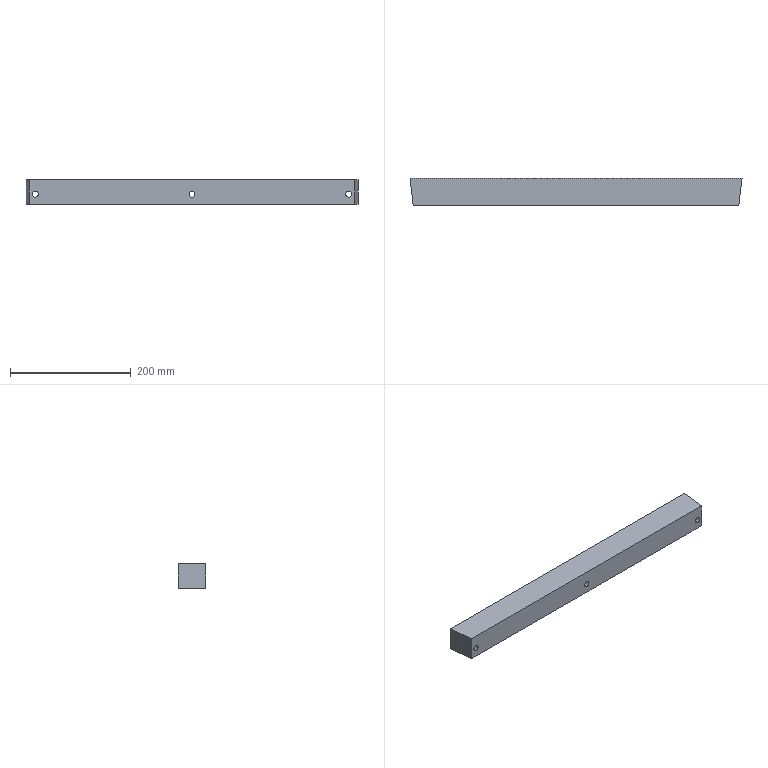Part | SolidWorks | features Extrusion 1, ICE 1 | 1 solid | 12 faces | box 550.66 x 45.55 x 40.5 mm | volume 995279 mm3 | cylinder 6 | plane 6 | commonest cylinder face diameters 10 x6
STEP:
#1=CARTESIAN_POINT('',(535.33,-45.55,-8.62));
#2=VERTEX_POINT('',#1);
#3=CARTESIAN_POINT('',(535.33,-45.55,1.38));
#4=VERTEX_POINT('',#3);
#5=CARTESIAN_POINT('',(535.33,-45.55,-3.62));
#6=DIRECTION('',(0.,1.,0.));
#7=DIRECTION('',(0.,0.,1.));
#8=AXIS2_PLACEMENT_3D('',#5,#6,#7);
#9=CIRCLE('',#8,5.);
#10=EDGE_CURVE('',#2,#4,#9,.T.);
#11=ORIENTED_EDGE('',*,*,#10,.F.);
#12=CARTESIAN_POINT('',(535.33,0.,-8.62));
#13=VERTEX_POINT('',#12);
#14=CARTESIAN_POINT('',(535.33,-52.5,-8.62));
#15=DIRECTION('',(0.,1.,0.));
#16=VECTOR('',#15,1000.);
#17=LINE('',#14,#16);
#18=EDGE_CURVE('',#2,#13,#17,.T.);
#19=ORIENTED_EDGE('',*,*,#18,.T.);
#20=CARTESIAN_POINT('',(535.33,0.,1.38));
#21=VERTEX_POINT('',#20);
#22=CARTESIAN_POINT('',(535.33,0.,-3.62));
#23=DIRECTION('',(0.,1.,0.));
#24=DIRECTION('',(0.,0.,1.));
#25=AXIS2_PLACEMENT_3D('',#22,#23,#24);
#26=CIRCLE('',#25,5.);
#27=EDGE_CURVE('',#13,#21,#26,.T.);
#28=ORIENTED_EDGE('',*,*,#27,.T.);
#29=CARTESIAN_POINT('',(535.33,-52.5,1.38));
#30=DIRECTION('',(0.,1.,0.));
#31=VECTOR('',#30,1000.);
#32=LINE('',#29,#31);
#33=EDGE_CURVE('',#4,#21,#32,.T.);
#34=ORIENTED_EDGE('',*,*,#33,.F.);
#35=EDGE_LOOP('',(#11,#19,#28,#34));
#36=FACE_OUTER_BOUND('',#35,.T.);
#37=CARTESIAN_POINT('',(535.33,-52.5,-3.62));
#38=DIRECTION('',(0.,1.,0.));
#39=DIRECTION('',(0.,0.,1.));
#40=AXIS2_PLACEMENT_3D('',#37,#38,#39);
#41=CYLINDRICAL_SURFACE('',#40,5.);
#42=ADVANCED_FACE('',(#36),#41,.F.);
#43=CARTESIAN_POINT('',(275.33,-45.55,-8.62));
#44=VERTEX_POINT('',#43);
#45=CARTESIAN_POINT('',(275.33,-45.55,1.38));
#46=VERTEX_POINT('',#45);
#47=CARTESIAN_POINT('',(275.33,-45.55,-3.62));
#48=DIRECTION('',(0.,1.,0.));
#49=DIRECTION('',(0.,0.,1.));
#50=AXIS2_PLACEMENT_3D('',#47,#48,#49);
#51=CIRCLE('',#50,5.);
#52=EDGE_CURVE('',#44,#46,#51,.T.);
#53=ORIENTED_EDGE('',*,*,#52,.F.);
#54=CARTESIAN_POINT('',(275.33,0.,-8.62));
#55=VERTEX_POINT('',#54);
#56=CARTESIAN_POINT('',(275.33,-52.5,-8.62));
#57=DIRECTION('',(0.,1.,0.));
#58=VECTOR('',#57,1000.);
#59=LINE('',#56,#58);
#60=EDGE_CURVE('',#44,#55,#59,.T.);
#61=ORIENTED_EDGE('',*,*,#60,.T.);
#62=CARTESIAN_POINT('',(275.33,0.,1.38));
#63=VERTEX_POINT('',#62);
#64=CARTESIAN_POINT('',(275.33,0.,-3.62));
#65=DIRECTION('',(0.,1.,0.));
#66=DIRECTION('',(0.,0.,1.));
#67=AXIS2_PLACEMENT_3D('',#64,#65,#66);
#68=CIRCLE('',#67,5.);
#69=EDGE_CURVE('',#55,#63,#68,.T.);
#70=ORIENTED_EDGE('',*,*,#69,.T.);
#71=CARTESIAN_POINT('',(275.33,-52.5,1.38));
#72=DIRECTION('',(0.,1.,0.));
#73=VECTOR('',#72,1000.);
#74=LINE('',#71,#73);
#75=EDGE_CURVE('',#46,#63,#74,.T.);
#76=ORIENTED_EDGE('',*,*,#75,.F.);
#77=EDGE_LOOP('',(#53,#61,#70,#76));
#78=FACE_OUTER_BOUND('',#77,.T.);
#79=CARTESIAN_POINT('',(275.33,-52.5,-3.62));
#80=DIRECTION('',(0.,1.,0.));
#81=DIRECTION('',(0.,0.,1.));
#82=AXIS2_PLACEMENT_3D('',#79,#80,#81);
#83=CYLINDRICAL_SURFACE('',#82,5.);
#84=ADVANCED_FACE('',(#78),#83,.F.);
#85=CARTESIAN_POINT('',(15.33,-45.55,-8.62));
#86=VERTEX_POINT('',#85);
#87=CARTESIAN_POINT('',(15.33,-45.55,1.38));
#88=VERTEX_POINT('',#87);
#89=CARTESIAN_POINT('',(15.33,-45.55,-3.62));
#90=DIRECTION('',(0.,1.,0.));
#91=DIRECTION('',(0.,0.,1.));
#92=AXIS2_PLACEMENT_3D('',#89,#90,#91);
#93=CIRCLE('',#92,5.);
#94=EDGE_CURVE('',#86,#88,#93,.T.);
#95=ORIENTED_EDGE('',*,*,#94,.F.);
#96=CARTESIAN_POINT('',(15.33,0.,-8.62));
#97=VERTEX_POINT('',#96);
#98=CARTESIAN_POINT('',(15.33,-52.5,-8.62));
#99=DIRECTION('',(0.,1.,0.));
#100=VECTOR('',#99,1000.);
#101=LINE('',#98,#100);
#102=EDGE_CURVE('',#86,#97,#101,.T.);
#103=ORIENTED_EDGE('',*,*,#102,.T.);
#104=CARTESIAN_POINT('',(15.33,0.,1.38));
#105=VERTEX_POINT('',#104);
#106=CARTESIAN_POINT('',(15.33,0.,-3.62));
#107=DIRECTION('',(0.,1.,0.));
#108=DIRECTION('',(0.,0.,1.));
#109=AXIS2_PLACEMENT_3D('',#106,#107,#108);
#110=CIRCLE('',#109,5.);
#111=EDGE_CURVE('',#97,#105,#110,.T.);
#112=ORIENTED_EDGE('',*,*,#111,.T.);
#113=CARTESIAN_POINT('',(15.33,-52.5,1.38));
#114=DIRECTION('',(0.,1.,0.));
#115=VECTOR('',#114,1000.);
#116=LINE('',#113,#115);
#117=EDGE_CURVE('',#88,#105,#116,.T.);
#118=ORIENTED_EDGE('',*,*,#117,.F.);
#119=EDGE_LOOP('',(#95,#103,#112,#118));
#120=FACE_OUTER_BOUND('',#119,.T.);
#121=CARTESIAN_POINT('',(15.33,-52.5,-3.62));
#122=DIRECTION('',(0.,1.,0.));
#123=DIRECTION('',(0.,0.,1.));
#124=AXIS2_PLACEMENT_3D('',#121,#122,#123);
#125=CYLINDRICAL_SURFACE('',#124,5.);
#126=ADVANCED_FACE('',(#120),#125,.F.);
#127=CARTESIAN_POINT('',(0.,0.,-20.25));
#128=VERTEX_POINT('',#127);
#129=CARTESIAN_POINT('',(5.33,-45.55,-20.25));
#130=VERTEX_POINT('',#129);
#131=CARTESIAN_POINT('',(0.,0.,-20.25));
#132=DIRECTION('',(0.1162,-0.9932,0.));
#133=VECTOR('',#132,1000.);
#134=LINE('',#131,#133);
#135=EDGE_CURVE('',#128,#130,#134,.T.);
#136=ORIENTED_EDGE('',*,*,#135,.T.);
#137=CARTESIAN_POINT('',(5.33,-45.55,20.25));
#138=VERTEX_POINT('',#137);
#139=CARTESIAN_POINT('',(5.33,-45.55,20.25));
#140=DIRECTION('',(0.,0.,-1.));
#141=VECTOR('',#140,1000.);
#142=LINE('',#139,#141);
#143=EDGE_CURVE('',#138,#130,#142,.T.);
#144=ORIENTED_EDGE('',*,*,#143,.F.);
#145=CARTESIAN_POINT('',(0.,0.,20.25));
#146=VERTEX_POINT('',#145);
#147=CARTESIAN_POINT('',(0.,0.,20.25));
#148=DIRECTION('',(0.1162,-0.9932,0.));
#149=VECTOR('',#148,1000.);
#150=LINE('',#147,#149);
#151=EDGE_CURVE('',#146,#138,#150,.T.);
#152=ORIENTED_EDGE('',*,*,#151,.F.);
#153=CARTESIAN_POINT('',(0.,0.,20.25));
#154=DIRECTION('',(0.,0.,-1.));
#155=VECTOR('',#154,1000.);
#156=LINE('',#153,#155);
#157=EDGE_CURVE('',#146,#128,#156,.T.);
#158=ORIENTED_EDGE('',*,*,#157,.T.);
#159=EDGE_LOOP('',(#136,#144,#152,#158));
#160=FACE_OUTER_BOUND('',#159,.T.);
#161=CARTESIAN_POINT('',(0.,0.,20.25));
#162=DIRECTION('',(0.9932,0.1162,0.));
#163=DIRECTION('',(-0.1162,0.9932,0.));
#164=AXIS2_PLACEMENT_3D('',#161,#162,#163);
#165=PLANE('',#164);
#166=ADVANCED_FACE('',(#160),#165,.F.);
#167=CARTESIAN_POINT('',(535.33,-45.55,-3.62));
#168=DIRECTION('',(0.,1.,0.));
#169=DIRECTION('',(0.,0.,1.));
#170=AXIS2_PLACEMENT_3D('',#167,#168,#169);
#171=CIRCLE('',#170,5.);
#172=EDGE_CURVE('',#4,#2,#171,.T.);
#173=ORIENTED_EDGE('',*,*,#172,.T.);
#174=ORIENTED_EDGE('',*,*,#10,.T.);
#175=EDGE_LOOP('',(#173,#174));
#176=FACE_BOUND('',#175,.T.);
#177=CARTESIAN_POINT('',(275.33,-45.55,-3.62));
#178=DIRECTION('',(0.,1.,0.));
#179=DIRECTION('',(0.,0.,1.));
#180=AXIS2_PLACEMENT_3D('',#177,#178,#179);
#181=CIRCLE('',#180,5.);
#182=EDGE_CURVE('',#46,#44,#181,.T.);
#183=ORIENTED_EDGE('',*,*,#182,.T.);
#184=ORIENTED_EDGE('',*,*,#52,.T.);
#185=EDGE_LOOP('',(#183,#184));
#186=FACE_BOUND('',#185,.T.);
#187=CARTESIAN_POINT('',(15.33,-45.55,-3.62));
#188=DIRECTION('',(0.,1.,0.));
#189=DIRECTION('',(0.,0.,1.));
#190=AXIS2_PLACEMENT_3D('',#187,#188,#189);
#191=CIRCLE('',#190,5.);
#192=EDGE_CURVE('',#88,#86,#191,.T.);
#193=ORIENTED_EDGE('',*,*,#192,.T.);
#194=ORIENTED_EDGE('',*,*,#94,.T.);
#195=EDGE_LOOP('',(#193,#194));
#196=FACE_BOUND('',#195,.T.);
#197=CARTESIAN_POINT('',(545.33,-45.55,-20.25));
#198=VERTEX_POINT('',#197);
#199=CARTESIAN_POINT('',(275.33,-45.55,-20.25));
#200=DIRECTION('',(1.,0.,0.));
#201=VECTOR('',#200,1000.);
#202=LINE('',#199,#201);
#203=EDGE_CURVE('',#130,#198,#202,.T.);
#204=ORIENTED_EDGE('',*,*,#203,.T.);
#205=CARTESIAN_POINT('',(545.33,-45.55,20.25));
#206=VERTEX_POINT('',#205);
#207=CARTESIAN_POINT('',(545.33,-45.55,20.25));
#208=DIRECTION('',(0.,0.,-1.));
#209=VECTOR('',#208,1000.);
#210=LINE('',#207,#209);
#211=EDGE_CURVE('',#206,#198,#210,.T.);
#212=ORIENTED_EDGE('',*,*,#211,.F.);
#213=CARTESIAN_POINT('',(275.33,-45.55,20.25));
#214=DIRECTION('',(1.,0.,0.));
#215=VECTOR('',#214,1000.);
#216=LINE('',#213,#215);
#217=EDGE_CURVE('',#138,#206,#216,.T.);
#218=ORIENTED_EDGE('',*,*,#217,.F.);
#219=ORIENTED_EDGE('',*,*,#143,.T.);
#220=EDGE_LOOP('',(#204,#212,#218,#219));
#221=FACE_OUTER_BOUND('',#220,.T.);
#222=CARTESIAN_POINT('',(275.33,-45.55,20.25));
#223=DIRECTION('',(0.,1.,0.));
#224=DIRECTION('',(0.,0.,1.));
#225=AXIS2_PLACEMENT_3D('',#222,#223,#224);
#226=PLANE('',#225);
#227=ADVANCED_FACE('',(#176,#186,#196,#221),#226,.F.);
#228=CARTESIAN_POINT('',(550.66,0.,-20.25));
#229=VERTEX_POINT('',#228);
#230=CARTESIAN_POINT('',(550.66,0.,-20.25));
#231=DIRECTION('',(0.1162,0.9932,0.));
#232=VECTOR('',#231,1000.);
#233=LINE('',#230,#232);
#234=EDGE_CURVE('',#198,#229,#233,.T.);
#235=ORIENTED_EDGE('',*,*,#234,.T.);
#236=CARTESIAN_POINT('',(550.66,0.,20.25));
#237=VERTEX_POINT('',#236);
#238=CARTESIAN_POINT('',(550.66,0.,20.25));
#239=DIRECTION('',(0.,0.,-1.));
#240=VECTOR('',#239,1000.);
#241=LINE('',#238,#240);
#242=EDGE_CURVE('',#237,#229,#241,.T.);
#243=ORIENTED_EDGE('',*,*,#242,.F.);
#244=CARTESIAN_POINT('',(550.66,0.,20.25));
#245=DIRECTION('',(0.1162,0.9932,0.));
#246=VECTOR('',#245,1000.);
#247=LINE('',#244,#246);
#248=EDGE_CURVE('',#206,#237,#247,.T.);
#249=ORIENTED_EDGE('',*,*,#248,.F.);
#250=ORIENTED_EDGE('',*,*,#211,.T.);
#251=EDGE_LOOP('',(#235,#243,#249,#250));
#252=FACE_OUTER_BOUND('',#251,.T.);
#253=CARTESIAN_POINT('',(550.66,0.,20.25));
#254=DIRECTION('',(-0.9932,0.1162,0.));
#255=DIRECTION('',(-0.1162,-0.9932,0.));
#256=AXIS2_PLACEMENT_3D('',#253,#254,#255);
#257=PLANE('',#256);
#258=ADVANCED_FACE('',(#252),#257,.F.);
#259=CARTESIAN_POINT('',(535.33,0.,-3.62));
#260=DIRECTION('',(0.,1.,0.));
#261=DIRECTION('',(0.,0.,1.));
#262=AXIS2_PLACEMENT_3D('',#259,#260,#261);
#263=CIRCLE('',#262,5.);
#264=EDGE_CURVE('',#21,#13,#263,.T.);
#265=ORIENTED_EDGE('',*,*,#264,.F.);
#266=ORIENTED_EDGE('',*,*,#27,.F.);
#267=EDGE_LOOP('',(#265,#266));
#268=FACE_BOUND('',#267,.T.);
#269=CARTESIAN_POINT('',(275.33,0.,-3.62));
#270=DIRECTION('',(0.,1.,0.));
#271=DIRECTION('',(0.,0.,1.));
#272=AXIS2_PLACEMENT_3D('',#269,#270,#271);
#273=CIRCLE('',#272,5.);
#274=EDGE_CURVE('',#63,#55,#273,.T.);
#275=ORIENTED_EDGE('',*,*,#274,.F.);
#276=ORIENTED_EDGE('',*,*,#69,.F.);
#277=EDGE_LOOP('',(#275,#276));
#278=FACE_BOUND('',#277,.T.);
#279=CARTESIAN_POINT('',(15.33,0.,-3.62));
#280=DIRECTION('',(0.,1.,0.));
#281=DIRECTION('',(0.,0.,1.));
#282=AXIS2_PLACEMENT_3D('',#279,#280,#281);
#283=CIRCLE('',#282,5.);
#284=EDGE_CURVE('',#105,#97,#283,.T.);
#285=ORIENTED_EDGE('',*,*,#284,.F.);
#286=ORIENTED_EDGE('',*,*,#111,.F.);
#287=EDGE_LOOP('',(#285,#286));
#288=FACE_BOUND('',#287,.T.);
#289=CARTESIAN_POINT('',(0.,0.,-20.25));
#290=DIRECTION('',(-1.,0.,0.));
#291=VECTOR('',#290,1000.);
#292=LINE('',#289,#291);
#293=EDGE_CURVE('',#229,#128,#292,.T.);
#294=ORIENTED_EDGE('',*,*,#293,.T.);
#295=ORIENTED_EDGE('',*,*,#157,.F.);
#296=CARTESIAN_POINT('',(0.,0.,20.25));
#297=DIRECTION('',(-1.,0.,0.));
#298=VECTOR('',#297,1000.);
#299=LINE('',#296,#298);
#300=EDGE_CURVE('',#237,#146,#299,.T.);
#301=ORIENTED_EDGE('',*,*,#300,.F.);
#302=ORIENTED_EDGE('',*,*,#242,.T.);
#303=EDGE_LOOP('',(#294,#295,#301,#302));
#304=FACE_OUTER_BOUND('',#303,.T.);
#305=CARTESIAN_POINT('',(0.,0.,20.25));
#306=DIRECTION('',(0.,-1.,0.));
#307=DIRECTION('',(0.,0.,-1.));
#308=AXIS2_PLACEMENT_3D('',#305,#306,#307);
#309=PLANE('',#308);
#310=ADVANCED_FACE('',(#268,#278,#288,#304),#309,.F.);
#311=ORIENTED_EDGE('',*,*,#151,.T.);
#312=ORIENTED_EDGE('',*,*,#217,.T.);
#313=ORIENTED_EDGE('',*,*,#248,.T.);
#314=ORIENTED_EDGE('',*,*,#300,.T.);
#315=EDGE_LOOP('',(#311,#312,#313,#314));
#316=FACE_OUTER_BOUND('',#315,.T.);
#317=CARTESIAN_POINT('',(0.,0.,20.25));
#318=DIRECTION('',(0.,0.,-1.));
#319=DIRECTION('',(-1.,0.,0.));
#320=AXIS2_PLACEMENT_3D('',#317,#318,#319);
#321=PLANE('',#320);
#322=ADVANCED_FACE('',(#316),#321,.F.);
#323=ORIENTED_EDGE('',*,*,#135,.F.);
#324=ORIENTED_EDGE('',*,*,#293,.F.);
#325=ORIENTED_EDGE('',*,*,#234,.F.);
#326=ORIENTED_EDGE('',*,*,#203,.F.);
#327=EDGE_LOOP('',(#323,#324,#325,#326));
#328=FACE_OUTER_BOUND('',#327,.T.);
#329=CARTESIAN_POINT('',(0.,0.,-20.25));
#330=DIRECTION('',(0.,0.,-1.));
#331=DIRECTION('',(-1.,0.,0.));
#332=AXIS2_PLACEMENT_3D('',#329,#330,#331);
#333=PLANE('',#332);
#334=ADVANCED_FACE('',(#328),#333,.T.);
#335=ORIENTED_EDGE('',*,*,#102,.F.);
#336=ORIENTED_EDGE('',*,*,#192,.F.);
#337=ORIENTED_EDGE('',*,*,#117,.T.);
#338=ORIENTED_EDGE('',*,*,#284,.T.);
#339=EDGE_LOOP('',(#335,#336,#337,#338));
#340=FACE_OUTER_BOUND('',#339,.T.);
#341=CARTESIAN_POINT('',(15.33,-52.5,-3.62));
#342=DIRECTION('',(0.,1.,0.));
#343=DIRECTION('',(0.,0.,1.));
#344=AXIS2_PLACEMENT_3D('',#341,#342,#343);
#345=CYLINDRICAL_SURFACE('',#344,5.);
#346=ADVANCED_FACE('',(#340),#345,.F.);
#347=ORIENTED_EDGE('',*,*,#60,.F.);
#348=ORIENTED_EDGE('',*,*,#182,.F.);
#349=ORIENTED_EDGE('',*,*,#75,.T.);
#350=ORIENTED_EDGE('',*,*,#274,.T.);
#351=EDGE_LOOP('',(#347,#348,#349,#350));
#352=FACE_OUTER_BOUND('',#351,.T.);
#353=CARTESIAN_POINT('',(275.33,-52.5,-3.62));
#354=DIRECTION('',(0.,1.,0.));
#355=DIRECTION('',(0.,0.,1.));
#356=AXIS2_PLACEMENT_3D('',#353,#354,#355);
#357=CYLINDRICAL_SURFACE('',#356,5.);
#358=ADVANCED_FACE('',(#352),#357,.F.);
#359=ORIENTED_EDGE('',*,*,#18,.F.);
#360=ORIENTED_EDGE('',*,*,#172,.F.);
#361=ORIENTED_EDGE('',*,*,#33,.T.);
#362=ORIENTED_EDGE('',*,*,#264,.T.);
#363=EDGE_LOOP('',(#359,#360,#361,#362));
#364=FACE_OUTER_BOUND('',#363,.T.);
#365=CARTESIAN_POINT('',(535.33,-52.5,-3.62));
#366=DIRECTION('',(0.,1.,0.));
#367=DIRECTION('',(0.,0.,1.));
#368=AXIS2_PLACEMENT_3D('',#365,#366,#367);
#369=CYLINDRICAL_SURFACE('',#368,5.);
#370=ADVANCED_FACE('',(#364),#369,.F.);
#371=CLOSED_SHELL('',(#42,#84,#126,#166,#227,#258,#310,#322,#334,#346,#358,#370));
#372=MANIFOLD_SOLID_BREP('',#371);
#373=CARTESIAN_POINT('',(0.,0.,0.));
#374=DIRECTION('',(0.,0.,1.));
#375=DIRECTION('',(1.,0.,0.));
#376=AXIS2_PLACEMENT_3D('',#373,#374,#375);
#377=(LENGTH_UNIT()NAMED_UNIT(*)SI_UNIT(.MILLI.,.METRE.));
#378=UNCERTAINTY_MEASURE_WITH_UNIT(LENGTH_MEASURE(0.00001),#377,'','');
#379=(NAMED_UNIT(*)PLANE_ANGLE_UNIT()SI_UNIT($,.RADIAN.));
#380=(NAMED_UNIT(*)SI_UNIT($,.STERADIAN.)SOLID_ANGLE_UNIT());
#381=(GEOMETRIC_REPRESENTATION_CONTEXT(3)GLOBAL_UNCERTAINTY_ASSIGNED_CONTEXT((#378))GLOBAL_UNIT_ASSIGNED_CONTEXT((#377,#379,#380))REPRESENTATION_CONTEXT('',''));
#382=ADVANCED_BREP_SHAPE_REPRESENTATION('',(#372,#376),#381);